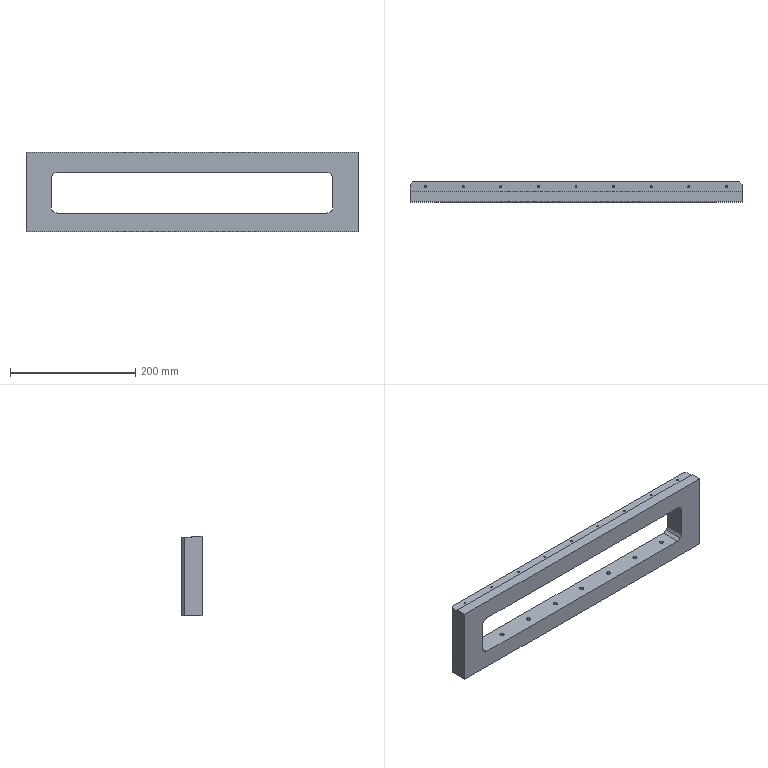Part | STEP file | ASND-0110-TCTF01-34 | 1 solid | 72 faces | box 530 x 32 x 127.1 mm | volume 1195079 mm3 | cylinder 40 | cone 18 | plane 14 | commonest cylinder face diameters 3 x18 6.5 x14 20 x8